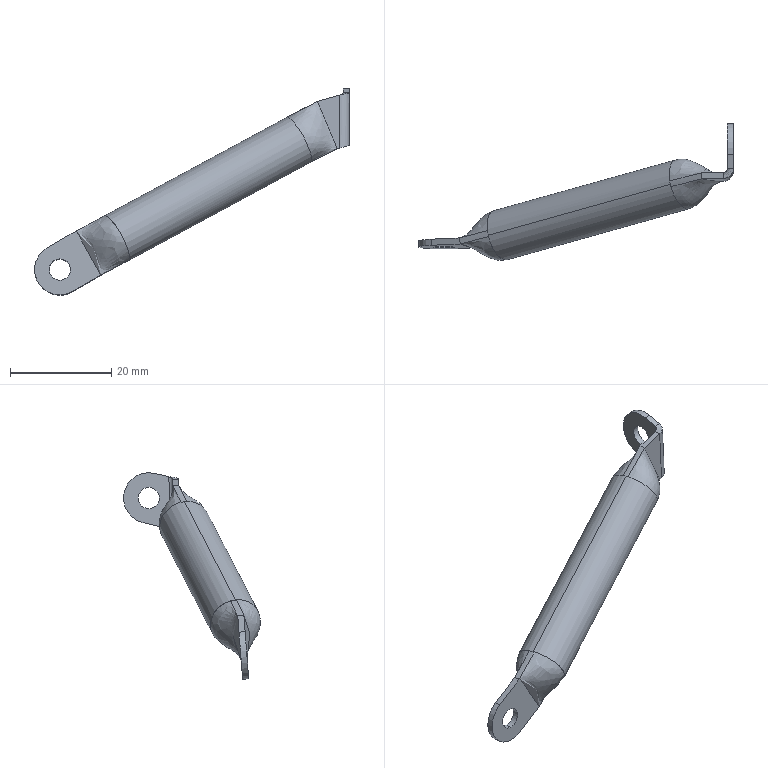Part | SolidWorks | features BaseBody 3 | 3 solids | 40 faces | box 62.052 x 26.99 x 40.735 mm | volume 1913 mm3 | plane 17 | cylinder 13 | spline 10 | commonest cylinder face diameters 10 x5 4.2 x4 8.4 x2 1.473 x1 3.873 x1